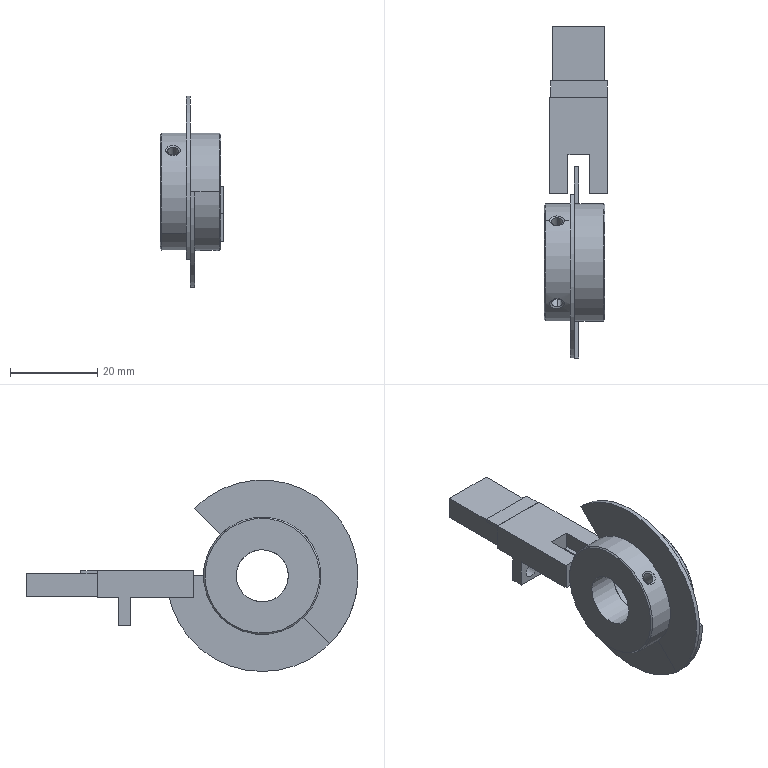Part | NX | 3 solids | 309 faces | box 14.7 x 76.3 x 44 mm | volume 10100 mm3 | plane 273 | cylinder 24 | spline 8 | cone 4 | commonest cylinder face diameters 2.5 x8 3.2 x4 12 x4 27 x4 1.6 x2 44 x2